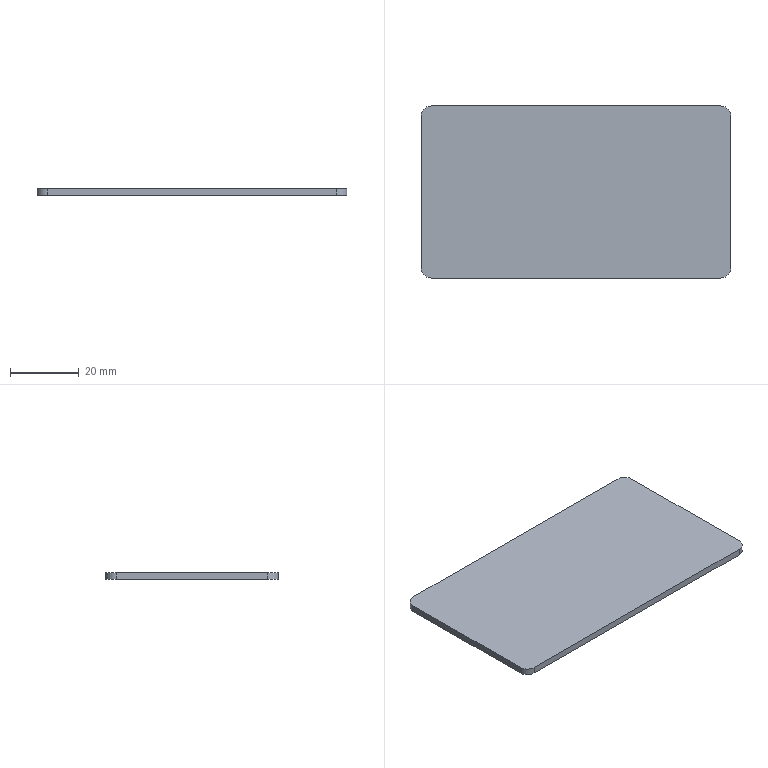Part | NX | features solid 2 | 1 solid | 10 faces | box 90 x 50 x 2 mm | volume 8985 mm3 | plane 6 | cylinder 4 | commonest cylinder face diameters 6 x4
STEP:
#1=CARTESIAN_POINT('',(-42.,124.,-81.5));
#2=VERTEX_POINT('',#1);
#3=CARTESIAN_POINT('',(42.,124.,-81.5));
#4=VERTEX_POINT('',#3);
#5=CARTESIAN_POINT('',(-0.000000019,124.,-81.5));
#6=DIRECTION('',(-1.,0.,-0.000000009));
#7=VECTOR('',#6,1000.);
#8=LINE('',#5,#7);
#9=EDGE_CURVE('',#2,#4,#8,.F.);
#10=ORIENTED_EDGE('',*,*,#9,.F.);
#11=CARTESIAN_POINT('',(-45.,121.,-81.5));
#12=VERTEX_POINT('',#11);
#13=CARTESIAN_POINT('',(-42.,121.,-81.5));
#14=DIRECTION('',(0.000000009,0.,-1.));
#15=DIRECTION('',(-1.,0.,-0.000000009));
#16=AXIS2_PLACEMENT_3D('',#13,#14,#15);
#17=CIRCLE('',#16,3.);
#18=EDGE_CURVE('',#2,#12,#17,.F.);
#19=ORIENTED_EDGE('',*,*,#18,.T.);
#20=CARTESIAN_POINT('',(-45.,77.,-81.5));
#21=VERTEX_POINT('',#20);
#22=CARTESIAN_POINT('',(-45.,99.,-81.5));
#23=DIRECTION('',(0.,-1.,0.));
#24=VECTOR('',#23,1000.);
#25=LINE('',#22,#24);
#26=EDGE_CURVE('',#21,#12,#25,.F.);
#27=ORIENTED_EDGE('',*,*,#26,.F.);
#28=CARTESIAN_POINT('',(-42.,74.,-81.5));
#29=VERTEX_POINT('',#28);
#30=CARTESIAN_POINT('',(-42.,77.,-81.5));
#31=DIRECTION('',(0.000000009,0.,-1.));
#32=DIRECTION('',(-1.,0.,-0.000000009));
#33=AXIS2_PLACEMENT_3D('',#30,#31,#32);
#34=CIRCLE('',#33,3.);
#35=EDGE_CURVE('',#21,#29,#34,.F.);
#36=ORIENTED_EDGE('',*,*,#35,.T.);
#37=CARTESIAN_POINT('',(42.,74.,-81.5));
#38=VERTEX_POINT('',#37);
#39=CARTESIAN_POINT('',(-0.000000019,74.,-81.5));
#40=DIRECTION('',(1.,0.,0.000000009));
#41=VECTOR('',#40,1000.);
#42=LINE('',#39,#41);
#43=EDGE_CURVE('',#38,#29,#42,.F.);
#44=ORIENTED_EDGE('',*,*,#43,.F.);
#45=CARTESIAN_POINT('',(45.,77.,-81.5));
#46=VERTEX_POINT('',#45);
#47=CARTESIAN_POINT('',(42.,77.,-81.5));
#48=DIRECTION('',(0.000000009,0.,-1.));
#49=DIRECTION('',(-1.,0.,-0.000000009));
#50=AXIS2_PLACEMENT_3D('',#47,#48,#49);
#51=CIRCLE('',#50,3.);
#52=EDGE_CURVE('',#38,#46,#51,.F.);
#53=ORIENTED_EDGE('',*,*,#52,.T.);
#54=CARTESIAN_POINT('',(45.,121.,-81.5));
#55=VERTEX_POINT('',#54);
#56=CARTESIAN_POINT('',(45.,99.,-81.5));
#57=DIRECTION('',(0.,1.,0.));
#58=VECTOR('',#57,1000.);
#59=LINE('',#56,#58);
#60=EDGE_CURVE('',#55,#46,#59,.F.);
#61=ORIENTED_EDGE('',*,*,#60,.F.);
#62=CARTESIAN_POINT('',(42.,121.,-81.5));
#63=DIRECTION('',(0.000000009,0.,-1.));
#64=DIRECTION('',(-1.,0.,-0.000000009));
#65=AXIS2_PLACEMENT_3D('',#62,#63,#64);
#66=CIRCLE('',#65,3.);
#67=EDGE_CURVE('',#55,#4,#66,.F.);
#68=ORIENTED_EDGE('',*,*,#67,.T.);
#69=EDGE_LOOP('',(#10,#19,#27,#36,#44,#53,#61,#68));
#70=FACE_BOUND('',#69,.T.);
#71=CARTESIAN_POINT('',(15.,99.3,-81.5));
#72=DIRECTION('',(0.000000009,0.,-1.));
#73=DIRECTION('',(0.,1.,0.));
#74=AXIS2_PLACEMENT_3D('',#71,#72,#73);
#75=PLANE('',#74);
#76=ADVANCED_FACE('',(#70),#75,.F.);
#77=CARTESIAN_POINT('',(45.,77.,-83.5));
#78=VERTEX_POINT('',#77);
#79=CARTESIAN_POINT('',(45.,121.,-83.5));
#80=VERTEX_POINT('',#79);
#81=CARTESIAN_POINT('',(45.,99.,-83.5));
#82=DIRECTION('',(0.,1.,0.));
#83=VECTOR('',#82,1000.);
#84=LINE('',#81,#83);
#85=EDGE_CURVE('',#78,#80,#84,.T.);
#86=ORIENTED_EDGE('',*,*,#85,.T.);
#87=CARTESIAN_POINT('',(45.,121.,-83.5));
#88=DIRECTION('',(0.,0.,1.));
#89=VECTOR('',#88,1000.);
#90=LINE('',#87,#89);
#91=EDGE_CURVE('',#80,#55,#90,.T.);
#92=ORIENTED_EDGE('',*,*,#91,.T.);
#93=ORIENTED_EDGE('',*,*,#60,.T.);
#94=CARTESIAN_POINT('',(45.,77.,-83.5));
#95=DIRECTION('',(0.,0.,1.));
#96=VECTOR('',#95,1000.);
#97=LINE('',#94,#96);
#98=EDGE_CURVE('',#46,#78,#97,.F.);
#99=ORIENTED_EDGE('',*,*,#98,.T.);
#100=EDGE_LOOP('',(#86,#92,#93,#99));
#101=FACE_BOUND('',#100,.T.);
#102=CARTESIAN_POINT('',(45.,99.,-83.5));
#103=DIRECTION('',(1.,0.,0.));
#104=DIRECTION('',(0.,0.,-1.));
#105=AXIS2_PLACEMENT_3D('',#102,#103,#104);
#106=PLANE('',#105);
#107=ADVANCED_FACE('',(#101),#106,.T.);
#108=ORIENTED_EDGE('',*,*,#43,.T.);
#109=CARTESIAN_POINT('',(-42.,74.,-83.5));
#110=VERTEX_POINT('',#109);
#111=CARTESIAN_POINT('',(-42.,74.,-83.5));
#112=DIRECTION('',(0.,0.,1.));
#113=VECTOR('',#112,1000.);
#114=LINE('',#111,#113);
#115=EDGE_CURVE('',#29,#110,#114,.F.);
#116=ORIENTED_EDGE('',*,*,#115,.T.);
#117=CARTESIAN_POINT('',(42.,74.,-83.5));
#118=VERTEX_POINT('',#117);
#119=CARTESIAN_POINT('',(0.,74.,-83.5));
#120=DIRECTION('',(1.,0.,0.000000009));
#121=VECTOR('',#120,1000.);
#122=LINE('',#119,#121);
#123=EDGE_CURVE('',#110,#118,#122,.T.);
#124=ORIENTED_EDGE('',*,*,#123,.T.);
#125=CARTESIAN_POINT('',(42.,74.,-83.5));
#126=DIRECTION('',(0.,0.,1.));
#127=VECTOR('',#126,1000.);
#128=LINE('',#125,#127);
#129=EDGE_CURVE('',#118,#38,#128,.T.);
#130=ORIENTED_EDGE('',*,*,#129,.T.);
#131=EDGE_LOOP('',(#108,#116,#124,#130));
#132=FACE_BOUND('',#131,.T.);
#133=CARTESIAN_POINT('',(0.,74.,-83.5));
#134=DIRECTION('',(0.,-1.,0.));
#135=DIRECTION('',(0.,0.,1.));
#136=AXIS2_PLACEMENT_3D('',#133,#134,#135);
#137=PLANE('',#136);
#138=ADVANCED_FACE('',(#132),#137,.T.);
#139=ORIENTED_EDGE('',*,*,#26,.T.);
#140=CARTESIAN_POINT('',(-45.,121.,-83.5));
#141=VERTEX_POINT('',#140);
#142=CARTESIAN_POINT('',(-45.,121.,-83.5));
#143=DIRECTION('',(0.,0.,1.));
#144=VECTOR('',#143,1000.);
#145=LINE('',#142,#144);
#146=EDGE_CURVE('',#12,#141,#145,.F.);
#147=ORIENTED_EDGE('',*,*,#146,.T.);
#148=CARTESIAN_POINT('',(-45.,77.,-83.5));
#149=VERTEX_POINT('',#148);
#150=CARTESIAN_POINT('',(-45.,99.,-83.5));
#151=DIRECTION('',(0.,-1.,0.));
#152=VECTOR('',#151,1000.);
#153=LINE('',#150,#152);
#154=EDGE_CURVE('',#141,#149,#153,.T.);
#155=ORIENTED_EDGE('',*,*,#154,.T.);
#156=CARTESIAN_POINT('',(-45.,77.,-83.5));
#157=DIRECTION('',(0.,0.,1.));
#158=VECTOR('',#157,1000.);
#159=LINE('',#156,#158);
#160=EDGE_CURVE('',#149,#21,#159,.T.);
#161=ORIENTED_EDGE('',*,*,#160,.T.);
#162=EDGE_LOOP('',(#139,#147,#155,#161));
#163=FACE_BOUND('',#162,.T.);
#164=CARTESIAN_POINT('',(-45.,99.,-83.5));
#165=DIRECTION('',(-1.,0.,0.));
#166=DIRECTION('',(0.,0.,1.));
#167=AXIS2_PLACEMENT_3D('',#164,#165,#166);
#168=PLANE('',#167);
#169=ADVANCED_FACE('',(#163),#168,.T.);
#170=ORIENTED_EDGE('',*,*,#154,.F.);
#171=CARTESIAN_POINT('',(-42.,124.,-83.5));
#172=VERTEX_POINT('',#171);
#173=CARTESIAN_POINT('',(-42.,121.,-83.5));
#174=DIRECTION('',(0.000000009,0.,-1.));
#175=DIRECTION('',(-1.,0.,-0.000000009));
#176=AXIS2_PLACEMENT_3D('',#173,#174,#175);
#177=CIRCLE('',#176,3.);
#178=EDGE_CURVE('',#141,#172,#177,.T.);
#179=ORIENTED_EDGE('',*,*,#178,.T.);
#180=CARTESIAN_POINT('',(42.,124.,-83.5));
#181=VERTEX_POINT('',#180);
#182=CARTESIAN_POINT('',(0.,124.,-83.5));
#183=DIRECTION('',(-1.,0.,-0.000000009));
#184=VECTOR('',#183,1000.);
#185=LINE('',#182,#184);
#186=EDGE_CURVE('',#181,#172,#185,.T.);
#187=ORIENTED_EDGE('',*,*,#186,.F.);
#188=CARTESIAN_POINT('',(42.,121.,-83.5));
#189=DIRECTION('',(0.000000009,0.,-1.));
#190=DIRECTION('',(-1.,0.,-0.000000009));
#191=AXIS2_PLACEMENT_3D('',#188,#189,#190);
#192=CIRCLE('',#191,3.);
#193=EDGE_CURVE('',#181,#80,#192,.T.);
#194=ORIENTED_EDGE('',*,*,#193,.T.);
#195=ORIENTED_EDGE('',*,*,#85,.F.);
#196=CARTESIAN_POINT('',(42.,77.,-83.5));
#197=DIRECTION('',(0.000000009,0.,-1.));
#198=DIRECTION('',(-1.,0.,-0.000000009));
#199=AXIS2_PLACEMENT_3D('',#196,#197,#198);
#200=CIRCLE('',#199,3.);
#201=EDGE_CURVE('',#78,#118,#200,.T.);
#202=ORIENTED_EDGE('',*,*,#201,.T.);
#203=ORIENTED_EDGE('',*,*,#123,.F.);
#204=CARTESIAN_POINT('',(-42.,77.,-83.5));
#205=DIRECTION('',(0.000000009,0.,-1.));
#206=DIRECTION('',(-1.,0.,-0.000000009));
#207=AXIS2_PLACEMENT_3D('',#204,#205,#206);
#208=CIRCLE('',#207,3.);
#209=EDGE_CURVE('',#110,#149,#208,.T.);
#210=ORIENTED_EDGE('',*,*,#209,.T.);
#211=EDGE_LOOP('',(#170,#179,#187,#194,#195,#202,#203,#210));
#212=FACE_BOUND('',#211,.T.);
#213=CARTESIAN_POINT('',(15.,99.3,-83.5));
#214=DIRECTION('',(0.000000009,0.,-1.));
#215=DIRECTION('',(0.,1.,0.));
#216=AXIS2_PLACEMENT_3D('',#213,#214,#215);
#217=PLANE('',#216);
#218=ADVANCED_FACE('',(#212),#217,.T.);
#219=ORIENTED_EDGE('',*,*,#186,.T.);
#220=CARTESIAN_POINT('',(-42.,124.,-83.5));
#221=DIRECTION('',(0.,0.,1.));
#222=VECTOR('',#221,1000.);
#223=LINE('',#220,#222);
#224=EDGE_CURVE('',#172,#2,#223,.T.);
#225=ORIENTED_EDGE('',*,*,#224,.T.);
#226=ORIENTED_EDGE('',*,*,#9,.T.);
#227=CARTESIAN_POINT('',(42.,124.,-83.5));
#228=DIRECTION('',(0.,0.,1.));
#229=VECTOR('',#228,1000.);
#230=LINE('',#227,#229);
#231=EDGE_CURVE('',#4,#181,#230,.F.);
#232=ORIENTED_EDGE('',*,*,#231,.T.);
#233=EDGE_LOOP('',(#219,#225,#226,#232));
#234=FACE_BOUND('',#233,.T.);
#235=CARTESIAN_POINT('',(0.,124.,-83.5));
#236=DIRECTION('',(0.,1.,0.));
#237=DIRECTION('',(0.,0.,-1.));
#238=AXIS2_PLACEMENT_3D('',#235,#236,#237);
#239=PLANE('',#238);
#240=ADVANCED_FACE('',(#234),#239,.T.);
#241=ORIENTED_EDGE('',*,*,#178,.F.);
#242=ORIENTED_EDGE('',*,*,#146,.F.);
#243=ORIENTED_EDGE('',*,*,#18,.F.);
#244=ORIENTED_EDGE('',*,*,#224,.F.);
#245=EDGE_LOOP('',(#241,#242,#243,#244));
#246=FACE_BOUND('',#245,.T.);
#247=CARTESIAN_POINT('',(-42.,121.,-83.5));
#248=DIRECTION('',(0.,0.,1.));
#249=DIRECTION('',(0.,1.,0.));
#250=AXIS2_PLACEMENT_3D('',#247,#248,#249);
#251=CYLINDRICAL_SURFACE('',#250,3.);
#252=ADVANCED_FACE('',(#246),#251,.T.);
#253=ORIENTED_EDGE('',*,*,#193,.F.);
#254=ORIENTED_EDGE('',*,*,#231,.F.);
#255=ORIENTED_EDGE('',*,*,#67,.F.);
#256=ORIENTED_EDGE('',*,*,#91,.F.);
#257=EDGE_LOOP('',(#253,#254,#255,#256));
#258=FACE_BOUND('',#257,.T.);
#259=CARTESIAN_POINT('',(42.,121.,-83.5));
#260=DIRECTION('',(0.,0.,1.));
#261=DIRECTION('',(0.,1.,0.));
#262=AXIS2_PLACEMENT_3D('',#259,#260,#261);
#263=CYLINDRICAL_SURFACE('',#262,3.);
#264=ADVANCED_FACE('',(#258),#263,.T.);
#265=ORIENTED_EDGE('',*,*,#209,.F.);
#266=ORIENTED_EDGE('',*,*,#115,.F.);
#267=ORIENTED_EDGE('',*,*,#35,.F.);
#268=ORIENTED_EDGE('',*,*,#160,.F.);
#269=EDGE_LOOP('',(#265,#266,#267,#268));
#270=FACE_BOUND('',#269,.T.);
#271=CARTESIAN_POINT('',(-42.,77.,-83.5));
#272=DIRECTION('',(0.,0.,1.));
#273=DIRECTION('',(0.,1.,0.));
#274=AXIS2_PLACEMENT_3D('',#271,#272,#273);
#275=CYLINDRICAL_SURFACE('',#274,3.);
#276=ADVANCED_FACE('',(#270),#275,.T.);
#277=ORIENTED_EDGE('',*,*,#201,.F.);
#278=ORIENTED_EDGE('',*,*,#98,.F.);
#279=ORIENTED_EDGE('',*,*,#52,.F.);
#280=ORIENTED_EDGE('',*,*,#129,.F.);
#281=EDGE_LOOP('',(#277,#278,#279,#280));
#282=FACE_BOUND('',#281,.T.);
#283=CARTESIAN_POINT('',(42.,77.,-83.5));
#284=DIRECTION('',(0.,0.,1.));
#285=DIRECTION('',(0.,1.,0.));
#286=AXIS2_PLACEMENT_3D('',#283,#284,#285);
#287=CYLINDRICAL_SURFACE('',#286,3.);
#288=ADVANCED_FACE('',(#282),#287,.T.);
#289=CLOSED_SHELL('',(#76,#107,#138,#169,#218,#240,#252,#264,#276,#288));
#290=MANIFOLD_SOLID_BREP('',#289);
#291=(LENGTH_UNIT()NAMED_UNIT(*)SI_UNIT(.MILLI.,.METRE.));
#292=UNCERTAINTY_MEASURE_WITH_UNIT(LENGTH_MEASURE(0.00001),#291,'','');
#293=(NAMED_UNIT(*)PLANE_ANGLE_UNIT()SI_UNIT($,.RADIAN.));
#294=(NAMED_UNIT(*)SI_UNIT($,.STERADIAN.)SOLID_ANGLE_UNIT());
#295=(GEOMETRIC_REPRESENTATION_CONTEXT(3)GLOBAL_UNCERTAINTY_ASSIGNED_CONTEXT((#292))GLOBAL_UNIT_ASSIGNED_CONTEXT((#291,#293,#294))REPRESENTATION_CONTEXT('',''));
#296=ADVANCED_BREP_SHAPE_REPRESENTATION('',(#290),#295);